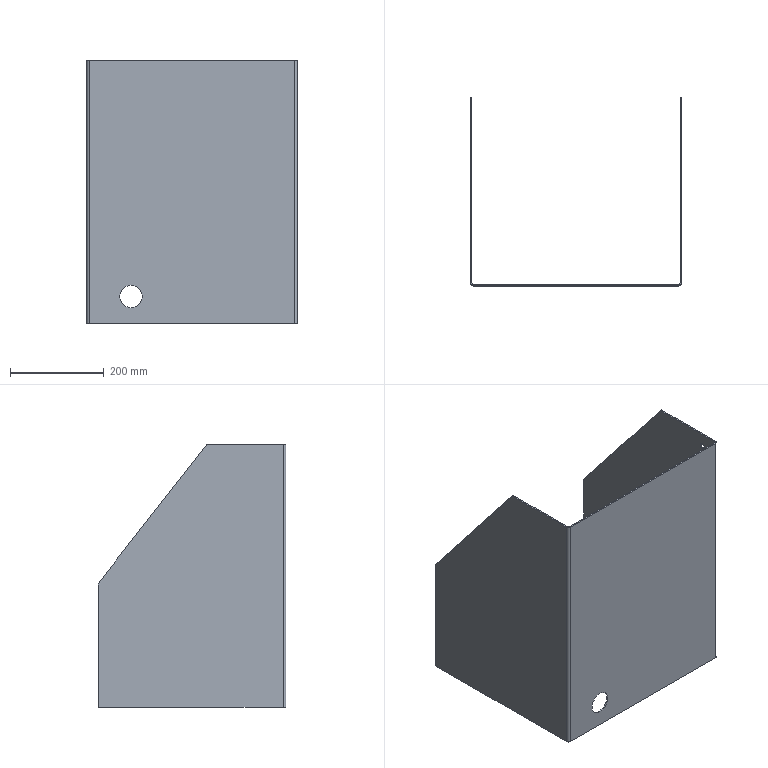Part | SolidWorks | features ICE 2, Cut 1, FlatPattern 1, SMBaseFlange 1, SheetMetal 1 | 1 solid | 36 faces | box 450 x 401 x 560 mm | volume 1875203 mm3 | plane 20 | cylinder 16 | commonest cylinder face diameters 6 x8 12.5 x4 12 x2 48 x2
STEP:
#1=CARTESIAN_POINT('',(95.,3.,33.));
#2=VERTEX_POINT('',#1);
#3=CARTESIAN_POINT('',(95.,3.,81.));
#4=VERTEX_POINT('',#3);
#5=CARTESIAN_POINT('',(95.,3.,57.));
#6=DIRECTION('',(0.,1.,0.));
#7=DIRECTION('',(0.,0.,1.));
#8=AXIS2_PLACEMENT_3D('',#5,#6,#7);
#9=CIRCLE('',#8,24.);
#10=EDGE_CURVE('',#2,#4,#9,.T.);
#11=ORIENTED_EDGE('',*,*,#10,.T.);
#12=CARTESIAN_POINT('',(95.,0.,81.));
#13=VERTEX_POINT('',#12);
#14=CARTESIAN_POINT('',(95.,10.,81.));
#15=DIRECTION('',(0.,-1.,0.));
#16=VECTOR('',#15,1000.);
#17=LINE('',#14,#16);
#18=EDGE_CURVE('',#4,#13,#17,.T.);
#19=ORIENTED_EDGE('',*,*,#18,.T.);
#20=CARTESIAN_POINT('',(95.,0.,33.));
#21=VERTEX_POINT('',#20);
#22=CARTESIAN_POINT('',(95.,0.,57.));
#23=DIRECTION('',(0.,-1.,0.));
#24=DIRECTION('',(0.,0.,-1.));
#25=AXIS2_PLACEMENT_3D('',#22,#23,#24);
#26=CIRCLE('',#25,24.);
#27=EDGE_CURVE('',#13,#21,#26,.T.);
#28=ORIENTED_EDGE('',*,*,#27,.T.);
#29=CARTESIAN_POINT('',(95.,10.,33.));
#30=DIRECTION('',(0.,-1.,0.));
#31=VECTOR('',#30,1000.);
#32=LINE('',#29,#31);
#33=EDGE_CURVE('',#2,#21,#32,.T.);
#34=ORIENTED_EDGE('',*,*,#33,.F.);
#35=EDGE_LOOP('',(#11,#19,#28,#34));
#36=FACE_OUTER_BOUND('',#35,.T.);
#37=CARTESIAN_POINT('',(95.,10.,57.));
#38=DIRECTION('',(0.,-1.,0.));
#39=DIRECTION('',(0.,0.,-1.));
#40=AXIS2_PLACEMENT_3D('',#37,#38,#39);
#41=CYLINDRICAL_SURFACE('',#40,24.);
#42=ADVANCED_FACE('',(#36),#41,.F.);
#43=CARTESIAN_POINT('',(447.,43.,373.75));
#44=VERTEX_POINT('',#43);
#45=CARTESIAN_POINT('',(447.,43.,386.25));
#46=VERTEX_POINT('',#45);
#47=CARTESIAN_POINT('',(447.,43.,380.));
#48=DIRECTION('',(-1.,0.,0.));
#49=DIRECTION('',(0.,0.,1.));
#50=AXIS2_PLACEMENT_3D('',#47,#48,#49);
#51=CIRCLE('',#50,6.25);
#52=EDGE_CURVE('',#44,#46,#51,.T.);
#53=ORIENTED_EDGE('',*,*,#52,.T.);
#54=CARTESIAN_POINT('',(450.,43.,386.25));
#55=VERTEX_POINT('',#54);
#56=CARTESIAN_POINT('',(440.,43.,386.25));
#57=DIRECTION('',(1.,0.,0.));
#58=VECTOR('',#57,1000.);
#59=LINE('',#56,#58);
#60=EDGE_CURVE('',#46,#55,#59,.T.);
#61=ORIENTED_EDGE('',*,*,#60,.T.);
#62=CARTESIAN_POINT('',(450.,43.,373.75));
#63=VERTEX_POINT('',#62);
#64=CARTESIAN_POINT('',(450.,43.,380.));
#65=DIRECTION('',(1.,0.,0.));
#66=DIRECTION('',(0.,0.,-1.));
#67=AXIS2_PLACEMENT_3D('',#64,#65,#66);
#68=CIRCLE('',#67,6.25);
#69=EDGE_CURVE('',#55,#63,#68,.T.);
#70=ORIENTED_EDGE('',*,*,#69,.T.);
#71=CARTESIAN_POINT('',(440.,43.,373.75));
#72=DIRECTION('',(1.,0.,0.));
#73=VECTOR('',#72,1000.);
#74=LINE('',#71,#73);
#75=EDGE_CURVE('',#44,#63,#74,.T.);
#76=ORIENTED_EDGE('',*,*,#75,.F.);
#77=EDGE_LOOP('',(#53,#61,#70,#76));
#78=FACE_OUTER_BOUND('',#77,.T.);
#79=CARTESIAN_POINT('',(440.,43.,380.));
#80=DIRECTION('',(1.,0.,0.));
#81=DIRECTION('',(0.,0.,-1.));
#82=AXIS2_PLACEMENT_3D('',#79,#80,#81);
#83=CYLINDRICAL_SURFACE('',#82,6.25);
#84=ADVANCED_FACE('',(#78),#83,.F.);
#85=CARTESIAN_POINT('',(447.,43.,523.75));
#86=VERTEX_POINT('',#85);
#87=CARTESIAN_POINT('',(447.,43.,536.25));
#88=VERTEX_POINT('',#87);
#89=CARTESIAN_POINT('',(447.,43.,530.));
#90=DIRECTION('',(-1.,0.,0.));
#91=DIRECTION('',(0.,0.,1.));
#92=AXIS2_PLACEMENT_3D('',#89,#90,#91);
#93=CIRCLE('',#92,6.25);
#94=EDGE_CURVE('',#86,#88,#93,.T.);
#95=ORIENTED_EDGE('',*,*,#94,.T.);
#96=CARTESIAN_POINT('',(450.,43.,536.25));
#97=VERTEX_POINT('',#96);
#98=CARTESIAN_POINT('',(440.,43.,536.25));
#99=DIRECTION('',(1.,0.,0.));
#100=VECTOR('',#99,1000.);
#101=LINE('',#98,#100);
#102=EDGE_CURVE('',#88,#97,#101,.T.);
#103=ORIENTED_EDGE('',*,*,#102,.T.);
#104=CARTESIAN_POINT('',(450.,43.,523.75));
#105=VERTEX_POINT('',#104);
#106=CARTESIAN_POINT('',(450.,43.,530.));
#107=DIRECTION('',(1.,0.,0.));
#108=DIRECTION('',(0.,0.,-1.));
#109=AXIS2_PLACEMENT_3D('',#106,#107,#108);
#110=CIRCLE('',#109,6.25);
#111=EDGE_CURVE('',#97,#105,#110,.T.);
#112=ORIENTED_EDGE('',*,*,#111,.T.);
#113=CARTESIAN_POINT('',(440.,43.,523.75));
#114=DIRECTION('',(1.,0.,0.));
#115=VECTOR('',#114,1000.);
#116=LINE('',#113,#115);
#117=EDGE_CURVE('',#86,#105,#116,.T.);
#118=ORIENTED_EDGE('',*,*,#117,.F.);
#119=EDGE_LOOP('',(#95,#103,#112,#118));
#120=FACE_OUTER_BOUND('',#119,.T.);
#121=CARTESIAN_POINT('',(440.,43.,530.));
#122=DIRECTION('',(1.,0.,0.));
#123=DIRECTION('',(0.,0.,-1.));
#124=AXIS2_PLACEMENT_3D('',#121,#122,#123);
#125=CYLINDRICAL_SURFACE('',#124,6.25);
#126=ADVANCED_FACE('',(#120),#125,.F.);
#127=CARTESIAN_POINT('',(450.,43.,380.));
#128=DIRECTION('',(1.,0.,0.));
#129=DIRECTION('',(0.,0.,-1.));
#130=AXIS2_PLACEMENT_3D('',#127,#128,#129);
#131=CIRCLE('',#130,6.25);
#132=EDGE_CURVE('',#63,#55,#131,.T.);
#133=ORIENTED_EDGE('',*,*,#132,.F.);
#134=ORIENTED_EDGE('',*,*,#69,.F.);
#135=EDGE_LOOP('',(#133,#134));
#136=FACE_BOUND('',#135,.T.);
#137=CARTESIAN_POINT('',(450.,43.,530.));
#138=DIRECTION('',(1.,0.,0.));
#139=DIRECTION('',(0.,0.,-1.));
#140=AXIS2_PLACEMENT_3D('',#137,#138,#139);
#141=CIRCLE('',#140,6.25);
#142=EDGE_CURVE('',#105,#97,#141,.T.);
#143=ORIENTED_EDGE('',*,*,#142,.F.);
#144=ORIENTED_EDGE('',*,*,#111,.F.);
#145=EDGE_LOOP('',(#143,#144));
#146=FACE_BOUND('',#145,.T.);
#147=CARTESIAN_POINT('',(450.,398.,0.));
#148=VERTEX_POINT('',#147);
#149=CARTESIAN_POINT('',(450.,401.,3.));
#150=VERTEX_POINT('',#149);
#151=CARTESIAN_POINT('',(450.,398.,3.));
#152=DIRECTION('',(1.,0.,0.));
#153=DIRECTION('',(0.,0.,1.));
#154=AXIS2_PLACEMENT_3D('',#151,#152,#153);
#155=CIRCLE('',#154,3.);
#156=EDGE_CURVE('',#148,#150,#155,.T.);
#157=ORIENTED_EDGE('',*,*,#156,.T.);
#158=CARTESIAN_POINT('',(450.,401.,262.934));
#159=VERTEX_POINT('',#158);
#160=CARTESIAN_POINT('',(450.,401.,560.));
#161=DIRECTION('',(0.,0.,-1.));
#162=VECTOR('',#161,1000.);
#163=LINE('',#160,#162);
#164=EDGE_CURVE('',#159,#150,#163,.T.);
#165=ORIENTED_EDGE('',*,*,#164,.F.);
#166=CARTESIAN_POINT('',(450.,400.364,264.781));
#167=VERTEX_POINT('',#166);
#168=CARTESIAN_POINT('',(450.,398.,262.934));
#169=DIRECTION('',(1.,0.,0.));
#170=DIRECTION('',(0.,0.,1.));
#171=AXIS2_PLACEMENT_3D('',#168,#169,#170);
#172=CIRCLE('',#171,3.);
#173=EDGE_CURVE('',#159,#167,#172,.T.);
#174=ORIENTED_EDGE('',*,*,#173,.T.);
#175=CARTESIAN_POINT('',(450.,170.611,558.847));
#176=VERTEX_POINT('',#175);
#177=CARTESIAN_POINT('',(450.,105.382,642.335));
#178=DIRECTION('',(0.,-0.6157,0.788));
#179=VECTOR('',#178,1000.);
#180=LINE('',#177,#179);
#181=EDGE_CURVE('',#167,#176,#180,.T.);
#182=ORIENTED_EDGE('',*,*,#181,.T.);
#183=CARTESIAN_POINT('',(450.,168.247,560.));
#184=VERTEX_POINT('',#183);
#185=CARTESIAN_POINT('',(450.,168.247,557.));
#186=DIRECTION('',(1.,0.,0.));
#187=DIRECTION('',(0.,0.,1.));
#188=AXIS2_PLACEMENT_3D('',#185,#186,#187);
#189=CIRCLE('',#188,3.);
#190=EDGE_CURVE('',#176,#184,#189,.T.);
#191=ORIENTED_EDGE('',*,*,#190,.T.);
#192=CARTESIAN_POINT('',(450.,6.,560.));
#193=VERTEX_POINT('',#192);
#194=CARTESIAN_POINT('',(450.,0.,560.));
#195=DIRECTION('',(0.,1.,0.));
#196=VECTOR('',#195,1000.);
#197=LINE('',#194,#196);
#198=EDGE_CURVE('',#193,#184,#197,.T.);
#199=ORIENTED_EDGE('',*,*,#198,.F.);
#200=CARTESIAN_POINT('',(450.,6.,0.));
#201=VERTEX_POINT('',#200);
#202=CARTESIAN_POINT('',(450.,6.,560.));
#203=DIRECTION('',(0.,0.,-1.));
#204=VECTOR('',#203,1000.);
#205=LINE('',#202,#204);
#206=EDGE_CURVE('',#193,#201,#205,.T.);
#207=ORIENTED_EDGE('',*,*,#206,.T.);
#208=CARTESIAN_POINT('',(450.,0.,0.));
#209=DIRECTION('',(0.,1.,0.));
#210=VECTOR('',#209,1000.);
#211=LINE('',#208,#210);
#212=EDGE_CURVE('',#201,#148,#211,.T.);
#213=ORIENTED_EDGE('',*,*,#212,.T.);
#214=EDGE_LOOP('',(#157,#165,#174,#182,#191,#199,#207,#213));
#215=FACE_OUTER_BOUND('',#214,.T.);
#216=CARTESIAN_POINT('',(450.,0.,560.));
#217=DIRECTION('',(-1.,0.,0.));
#218=DIRECTION('',(0.,0.,1.));
#219=AXIS2_PLACEMENT_3D('',#216,#217,#218);
#220=PLANE('',#219);
#221=ADVANCED_FACE('',(#136,#146,#215),#220,.F.);
#222=ORIENTED_EDGE('',*,*,#52,.F.);
#223=CARTESIAN_POINT('',(447.,43.,380.));
#224=DIRECTION('',(-1.,0.,0.));
#225=DIRECTION('',(0.,0.,1.));
#226=AXIS2_PLACEMENT_3D('',#223,#224,#225);
#227=CIRCLE('',#226,6.25);
#228=EDGE_CURVE('',#46,#44,#227,.T.);
#229=ORIENTED_EDGE('',*,*,#228,.F.);
#230=EDGE_LOOP('',(#222,#229));
#231=FACE_BOUND('',#230,.T.);
#232=ORIENTED_EDGE('',*,*,#94,.F.);
#233=CARTESIAN_POINT('',(447.,43.,530.));
#234=DIRECTION('',(-1.,0.,0.));
#235=DIRECTION('',(0.,0.,1.));
#236=AXIS2_PLACEMENT_3D('',#233,#234,#235);
#237=CIRCLE('',#236,6.25);
#238=EDGE_CURVE('',#88,#86,#237,.T.);
#239=ORIENTED_EDGE('',*,*,#238,.F.);
#240=EDGE_LOOP('',(#232,#239));
#241=FACE_BOUND('',#240,.T.);
#242=CARTESIAN_POINT('',(447.,401.,262.934));
#243=VERTEX_POINT('',#242);
#244=CARTESIAN_POINT('',(447.,401.,3.));
#245=VERTEX_POINT('',#244);
#246=CARTESIAN_POINT('',(447.,401.,560.));
#247=DIRECTION('',(0.,0.,-1.));
#248=VECTOR('',#247,1000.);
#249=LINE('',#246,#248);
#250=EDGE_CURVE('',#243,#245,#249,.T.);
#251=ORIENTED_EDGE('',*,*,#250,.T.);
#252=CARTESIAN_POINT('',(447.,398.,0.));
#253=VERTEX_POINT('',#252);
#254=CARTESIAN_POINT('',(447.,398.,3.));
#255=DIRECTION('',(1.,0.,0.));
#256=DIRECTION('',(0.,0.,1.));
#257=AXIS2_PLACEMENT_3D('',#254,#255,#256);
#258=CIRCLE('',#257,3.);
#259=EDGE_CURVE('',#253,#245,#258,.T.);
#260=ORIENTED_EDGE('',*,*,#259,.F.);
#261=CARTESIAN_POINT('',(447.,6.,0.));
#262=VERTEX_POINT('',#261);
#263=CARTESIAN_POINT('',(447.,0.,0.));
#264=DIRECTION('',(0.,1.,0.));
#265=VECTOR('',#264,1000.);
#266=LINE('',#263,#265);
#267=EDGE_CURVE('',#262,#253,#266,.T.);
#268=ORIENTED_EDGE('',*,*,#267,.F.);
#269=CARTESIAN_POINT('',(447.,6.,560.));
#270=VERTEX_POINT('',#269);
#271=CARTESIAN_POINT('',(447.,6.,560.));
#272=DIRECTION('',(0.,0.,-1.));
#273=VECTOR('',#272,1000.);
#274=LINE('',#271,#273);
#275=EDGE_CURVE('',#270,#262,#274,.T.);
#276=ORIENTED_EDGE('',*,*,#275,.F.);
#277=CARTESIAN_POINT('',(447.,168.247,560.));
#278=VERTEX_POINT('',#277);
#279=CARTESIAN_POINT('',(447.,0.,560.));
#280=DIRECTION('',(0.,1.,0.));
#281=VECTOR('',#280,1000.);
#282=LINE('',#279,#281);
#283=EDGE_CURVE('',#270,#278,#282,.T.);
#284=ORIENTED_EDGE('',*,*,#283,.T.);
#285=CARTESIAN_POINT('',(447.,170.611,558.847));
#286=VERTEX_POINT('',#285);
#287=CARTESIAN_POINT('',(447.,168.247,557.));
#288=DIRECTION('',(1.,0.,0.));
#289=DIRECTION('',(0.,0.,1.));
#290=AXIS2_PLACEMENT_3D('',#287,#288,#289);
#291=CIRCLE('',#290,3.);
#292=EDGE_CURVE('',#286,#278,#291,.T.);
#293=ORIENTED_EDGE('',*,*,#292,.F.);
#294=CARTESIAN_POINT('',(447.,400.364,264.781));
#295=VERTEX_POINT('',#294);
#296=CARTESIAN_POINT('',(447.,105.382,642.335));
#297=DIRECTION('',(0.,-0.6157,0.788));
#298=VECTOR('',#297,1000.);
#299=LINE('',#296,#298);
#300=EDGE_CURVE('',#295,#286,#299,.T.);
#301=ORIENTED_EDGE('',*,*,#300,.F.);
#302=CARTESIAN_POINT('',(447.,398.,262.934));
#303=DIRECTION('',(1.,0.,0.));
#304=DIRECTION('',(0.,0.,1.));
#305=AXIS2_PLACEMENT_3D('',#302,#303,#304);
#306=CIRCLE('',#305,3.);
#307=EDGE_CURVE('',#243,#295,#306,.T.);
#308=ORIENTED_EDGE('',*,*,#307,.F.);
#309=EDGE_LOOP('',(#251,#260,#268,#276,#284,#293,#301,#308));
#310=FACE_OUTER_BOUND('',#309,.T.);
#311=CARTESIAN_POINT('',(447.,0.,560.));
#312=DIRECTION('',(-1.,0.,0.));
#313=DIRECTION('',(0.,0.,1.));
#314=AXIS2_PLACEMENT_3D('',#311,#312,#313);
#315=PLANE('',#314);
#316=ADVANCED_FACE('',(#231,#241,#310),#315,.T.);
#317=ORIENTED_EDGE('',*,*,#164,.T.);
#318=CARTESIAN_POINT('',(447.,401.,3.));
#319=DIRECTION('',(1.,0.,0.));
#320=VECTOR('',#319,1000.);
#321=LINE('',#318,#320);
#322=EDGE_CURVE('',#245,#150,#321,.T.);
#323=ORIENTED_EDGE('',*,*,#322,.F.);
#324=ORIENTED_EDGE('',*,*,#250,.F.);
#325=CARTESIAN_POINT('',(447.,401.,262.934));
#326=DIRECTION('',(1.,0.,0.));
#327=VECTOR('',#326,1000.);
#328=LINE('',#325,#327);
#329=EDGE_CURVE('',#243,#159,#328,.T.);
#330=ORIENTED_EDGE('',*,*,#329,.T.);
#331=EDGE_LOOP('',(#317,#323,#324,#330));
#332=FACE_OUTER_BOUND('',#331,.T.);
#333=CARTESIAN_POINT('',(447.,401.,560.));
#334=DIRECTION('',(0.,1.,0.));
#335=DIRECTION('',(0.,0.,1.));
#336=AXIS2_PLACEMENT_3D('',#333,#334,#335);
#337=PLANE('',#336);
#338=ADVANCED_FACE('',(#332),#337,.T.);
#339=CARTESIAN_POINT('',(3.,398.,0.));
#340=VERTEX_POINT('',#339);
#341=CARTESIAN_POINT('',(3.,6.,0.));
#342=VERTEX_POINT('',#341);
#343=CARTESIAN_POINT('',(3.,0.,0.));
#344=DIRECTION('',(0.,-1.,0.));
#345=VECTOR('',#344,1000.);
#346=LINE('',#343,#345);
#347=EDGE_CURVE('',#340,#342,#346,.T.);
#348=ORIENTED_EDGE('',*,*,#347,.F.);
#349=CARTESIAN_POINT('',(3.,401.,3.));
#350=VERTEX_POINT('',#349);
#351=CARTESIAN_POINT('',(3.,398.,3.));
#352=DIRECTION('',(-1.,0.,0.));
#353=DIRECTION('',(0.,0.,-1.));
#354=AXIS2_PLACEMENT_3D('',#351,#352,#353);
#355=CIRCLE('',#354,3.);
#356=EDGE_CURVE('',#350,#340,#355,.T.);
#357=ORIENTED_EDGE('',*,*,#356,.F.);
#358=CARTESIAN_POINT('',(3.,401.,262.934));
#359=VERTEX_POINT('',#358);
#360=CARTESIAN_POINT('',(3.,401.,560.));
#361=DIRECTION('',(0.,0.,-1.));
#362=VECTOR('',#361,1000.);
#363=LINE('',#360,#362);
#364=EDGE_CURVE('',#359,#350,#363,.T.);
#365=ORIENTED_EDGE('',*,*,#364,.F.);
#366=CARTESIAN_POINT('',(3.,400.364,264.781));
#367=VERTEX_POINT('',#366);
#368=CARTESIAN_POINT('',(3.,398.,262.934));
#369=DIRECTION('',(-1.,0.,0.));
#370=DIRECTION('',(0.,0.,-1.));
#371=AXIS2_PLACEMENT_3D('',#368,#369,#370);
#372=CIRCLE('',#371,3.);
#373=EDGE_CURVE('',#367,#359,#372,.T.);
#374=ORIENTED_EDGE('',*,*,#373,.F.);
#375=CARTESIAN_POINT('',(3.,170.611,558.847));
#376=VERTEX_POINT('',#375);
#377=CARTESIAN_POINT('',(3.,105.382,642.335));
#378=DIRECTION('',(0.,0.6157,-0.788));
#379=VECTOR('',#378,1000.);
#380=LINE('',#377,#379);
#381=EDGE_CURVE('',#376,#367,#380,.T.);
#382=ORIENTED_EDGE('',*,*,#381,.F.);
#383=CARTESIAN_POINT('',(3.,168.247,560.));
#384=VERTEX_POINT('',#383);
#385=CARTESIAN_POINT('',(3.,168.247,557.));
#386=DIRECTION('',(-1.,0.,0.));
#387=DIRECTION('',(0.,0.,-1.));
#388=AXIS2_PLACEMENT_3D('',#385,#386,#387);
#389=CIRCLE('',#388,3.);
#390=EDGE_CURVE('',#384,#376,#389,.T.);
#391=ORIENTED_EDGE('',*,*,#390,.F.);
#392=CARTESIAN_POINT('',(3.,6.,560.));
#393=VERTEX_POINT('',#392);
#394=CARTESIAN_POINT('',(3.,0.,560.));
#395=DIRECTION('',(0.,-1.,0.));
#396=VECTOR('',#395,1000.);
#397=LINE('',#394,#396);
#398=EDGE_CURVE('',#384,#393,#397,.T.);
#399=ORIENTED_EDGE('',*,*,#398,.T.);
#400=CARTESIAN_POINT('',(3.,6.,560.));
#401=DIRECTION('',(0.,0.,-1.));
#402=VECTOR('',#401,1000.);
#403=LINE('',#400,#402);
#404=EDGE_CURVE('',#393,#342,#403,.T.);
#405=ORIENTED_EDGE('',*,*,#404,.T.);
#406=EDGE_LOOP('',(#348,#357,#365,#374,#382,#391,#399,#405));
#407=FACE_OUTER_BOUND('',#406,.T.);
#408=CARTESIAN_POINT('',(3.,0.,560.));
#409=DIRECTION('',(1.,0.,0.));
#410=DIRECTION('',(0.,0.,-1.));
#411=AXIS2_PLACEMENT_3D('',#408,#409,#410);
#412=PLANE('',#411);
#413=ADVANCED_FACE('',(#407),#412,.T.);
#414=CARTESIAN_POINT('',(0.,401.,3.));
#415=VERTEX_POINT('',#414);
#416=CARTESIAN_POINT('',(0.,398.,0.));
#417=VERTEX_POINT('',#416);
#418=CARTESIAN_POINT('',(0.,398.,3.));
#419=DIRECTION('',(-1.,0.,0.));
#420=DIRECTION('',(0.,0.,-1.));
#421=AXIS2_PLACEMENT_3D('',#418,#419,#420);
#422=CIRCLE('',#421,3.);
#423=EDGE_CURVE('',#415,#417,#422,.T.);
#424=ORIENTED_EDGE('',*,*,#423,.T.);
#425=CARTESIAN_POINT('',(0.,6.,0.));
#426=VERTEX_POINT('',#425);
#427=CARTESIAN_POINT('',(0.,0.,0.));
#428=DIRECTION('',(0.,-1.,0.));
#429=VECTOR('',#428,1000.);
#430=LINE('',#427,#429);
#431=EDGE_CURVE('',#417,#426,#430,.T.);
#432=ORIENTED_EDGE('',*,*,#431,.T.);
#433=CARTESIAN_POINT('',(0.,6.,560.));
#434=VERTEX_POINT('',#433);
#435=CARTESIAN_POINT('',(0.,6.,560.));
#436=DIRECTION('',(0.,0.,-1.));
#437=VECTOR('',#436,1000.);
#438=LINE('',#435,#437);
#439=EDGE_CURVE('',#434,#426,#438,.T.);
#440=ORIENTED_EDGE('',*,*,#439,.F.);
#441=CARTESIAN_POINT('',(0.,168.247,560.));
#442=VERTEX_POINT('',#441);
#443=CARTESIAN_POINT('',(0.,0.,560.));
#444=DIRECTION('',(0.,-1.,0.));
#445=VECTOR('',#444,1000.);
#446=LINE('',#443,#445);
#447=EDGE_CURVE('',#442,#434,#446,.T.);
#448=ORIENTED_EDGE('',*,*,#447,.F.);
#449=CARTESIAN_POINT('',(0.,170.611,558.847));
#450=VERTEX_POINT('',#449);
#451=CARTESIAN_POINT('',(0.,168.247,557.));
#452=DIRECTION('',(-1.,0.,0.));
#453=DIRECTION('',(0.,0.,-1.));
#454=AXIS2_PLACEMENT_3D('',#451,#452,#453);
#455=CIRCLE('',#454,3.);
#456=EDGE_CURVE('',#442,#450,#455,.T.);
#457=ORIENTED_EDGE('',*,*,#456,.T.);
#458=CARTESIAN_POINT('',(0.,400.364,264.781));
#459=VERTEX_POINT('',#458);
#460=CARTESIAN_POINT('',(0.,105.382,642.335));
#461=DIRECTION('',(0.,0.6157,-0.788));
#462=VECTOR('',#461,1000.);
#463=LINE('',#460,#462);
#464=EDGE_CURVE('',#450,#459,#463,.T.);
#465=ORIENTED_EDGE('',*,*,#464,.T.);
#466=CARTESIAN_POINT('',(0.,401.,262.934));
#467=VERTEX_POINT('',#466);
#468=CARTESIAN_POINT('',(0.,398.,262.934));
#469=DIRECTION('',(-1.,0.,0.));
#470=DIRECTION('',(0.,0.,-1.));
#471=AXIS2_PLACEMENT_3D('',#468,#469,#470);
#472=CIRCLE('',#471,3.);
#473=EDGE_CURVE('',#459,#467,#472,.T.);
#474=ORIENTED_EDGE('',*,*,#473,.T.);
#475=CARTESIAN_POINT('',(0.,401.,560.));
#476=DIRECTION('',(0.,0.,-1.));
#477=VECTOR('',#476,1000.);
#478=LINE('',#475,#477);
#479=EDGE_CURVE('',#467,#415,#478,.T.);
#480=ORIENTED_EDGE('',*,*,#479,.T.);
#481=EDGE_LOOP('',(#424,#432,#440,#448,#457,#465,#474,#480));
#482=FACE_OUTER_BOUND('',#481,.T.);
#483=CARTESIAN_POINT('',(0.,0.,560.));
#484=DIRECTION('',(1.,0.,0.));
#485=DIRECTION('',(0.,0.,-1.));
#486=AXIS2_PLACEMENT_3D('',#483,#484,#485);
#487=PLANE('',#486);
#488=ADVANCED_FACE('',(#482),#487,.F.);
#489=ORIENTED_EDGE('',*,*,#198,.T.);
#490=CARTESIAN_POINT('',(447.,168.247,560.));
#491=DIRECTION('',(1.,0.,0.));
#492=VECTOR('',#491,1000.);
#493=LINE('',#490,#492);
#494=EDGE_CURVE('',#278,#184,#493,.T.);
#495=ORIENTED_EDGE('',*,*,#494,.F.);
#496=ORIENTED_EDGE('',*,*,#283,.F.);
#497=CARTESIAN_POINT('',(447.,6.,560.));
#498=DIRECTION('',(1.,0.,0.));
#499=VECTOR('',#498,1000.);
#500=LINE('',#497,#499);
#501=EDGE_CURVE('',#270,#193,#500,.T.);
#502=ORIENTED_EDGE('',*,*,#501,.T.);
#503=EDGE_LOOP('',(#489,#495,#496,#502));
#504=FACE_OUTER_BOUND('',#503,.T.);
#505=CARTESIAN_POINT('',(444.,6.,560.));
#506=DIRECTION('',(0.,0.,1.));
#507=DIRECTION('',(1.,0.,0.));
#508=AXIS2_PLACEMENT_3D('',#505,#506,#507);
#509=PLANE('',#508);
#510=ADVANCED_FACE('',(#504),#509,.T.);
#511=CARTESIAN_POINT('',(3.,401.,3.));
#512=DIRECTION('',(-1.,0.,0.));
#513=VECTOR('',#512,1000.);
#514=LINE('',#511,#513);
#515=EDGE_CURVE('',#350,#415,#514,.T.);
#516=ORIENTED_EDGE('',*,*,#515,.T.);
#517=ORIENTED_EDGE('',*,*,#479,.F.);
#518=CARTESIAN_POINT('',(3.,401.,262.934));
#519=DIRECTION('',(-1.,0.,0.));
#520=VECTOR('',#519,1000.);
#521=LINE('',#518,#520);
#522=EDGE_CURVE('',#359,#467,#521,.T.);
#523=ORIENTED_EDGE('',*,*,#522,.F.);
#524=ORIENTED_EDGE('',*,*,#364,.T.);
#525=EDGE_LOOP('',(#516,#517,#523,#524));
#526=FACE_OUTER_BOUND('',#525,.T.);
#527=CARTESIAN_POINT('',(0.,401.,560.));
#528=DIRECTION('',(0.,1.,0.));
#529=DIRECTION('',(0.,0.,1.));
#530=AXIS2_PLACEMENT_3D('',#527,#528,#529);
#531=PLANE('',#530);
#532=ADVANCED_FACE('',(#526),#531,.T.);
#533=CARTESIAN_POINT('',(0.,6.,560.));
#534=DIRECTION('',(1.,0.,0.));
#535=VECTOR('',#534,1000.);
#536=LINE('',#533,#535);
#537=EDGE_CURVE('',#434,#393,#536,.T.);
#538=ORIENTED_EDGE('',*,*,#537,.F.);
#539=CARTESIAN_POINT('',(6.,0.,560.));
#540=VERTEX_POINT('',#539);
#541=CARTESIAN_POINT('',(6.,6.,560.));
#542=DIRECTION('',(0.,0.,1.));
#543=DIRECTION('',(-1.,0.,0.));
#544=AXIS2_PLACEMENT_3D('',#541,#542,#543);
#545=CIRCLE('',#544,6.);
#546=EDGE_CURVE('',#434,#540,#545,.T.);
#547=ORIENTED_EDGE('',*,*,#546,.T.);
#548=CARTESIAN_POINT('',(6.,3.,560.));
#549=VERTEX_POINT('',#548);
#550=CARTESIAN_POINT('',(6.,3.,560.));
#551=DIRECTION('',(0.,-1.,0.));
#552=VECTOR('',#551,1000.);
#553=LINE('',#550,#552);
#554=EDGE_CURVE('',#549,#540,#553,.T.);
#555=ORIENTED_EDGE('',*,*,#554,.F.);
#556=CARTESIAN_POINT('',(6.,6.,560.));
#557=DIRECTION('',(0.,0.,1.));
#558=DIRECTION('',(1.,0.,0.));
#559=AXIS2_PLACEMENT_3D('',#556,#557,#558);
#560=CIRCLE('',#559,3.);
#561=EDGE_CURVE('',#393,#549,#560,.T.);
#562=ORIENTED_EDGE('',*,*,#561,.F.);
#563=EDGE_LOOP('',(#538,#547,#555,#562));
#564=FACE_OUTER_BOUND('',#563,.T.);
#565=CARTESIAN_POINT('',(0.,6.,560.));
#566=DIRECTION('',(0.,0.,1.));
#567=DIRECTION('',(1.,0.,0.));
#568=AXIS2_PLACEMENT_3D('',#565,#566,#567);
#569=PLANE('',#568);
#570=ADVANCED_FACE('',(#564),#569,.T.);
#571=CARTESIAN_POINT('',(3.,168.247,560.));
#572=DIRECTION('',(-1.,0.,0.));
#573=VECTOR('',#572,1000.);
#574=LINE('',#571,#573);
#575=EDGE_CURVE('',#384,#442,#574,.T.);
#576=ORIENTED_EDGE('',*,*,#575,.T.);
#577=ORIENTED_EDGE('',*,*,#447,.T.);
#578=ORIENTED_EDGE('',*,*,#537,.T.);
#579=ORIENTED_EDGE('',*,*,#398,.F.);
#580=EDGE_LOOP('',(#576,#577,#578,#579));
#581=FACE_OUTER_BOUND('',#580,.T.);
#582=CARTESIAN_POINT('',(6.,3.,560.));
#583=DIRECTION('',(0.,0.,1.));
#584=DIRECTION('',(1.,0.,0.));
#585=AXIS2_PLACEMENT_3D('',#582,#583,#584);
#586=PLANE('',#585);
#587=ADVANCED_FACE('',(#581),#586,.T.);
#588=CARTESIAN_POINT('',(6.,0.,0.));
#589=VERTEX_POINT('',#588);
#590=CARTESIAN_POINT('',(6.,3.,0.));
#591=VERTEX_POINT('',#590);
#592=CARTESIAN_POINT('',(6.,0.,0.));
#593=DIRECTION('',(0.,1.,0.));
#594=VECTOR('',#593,1000.);
#595=LINE('',#592,#594);
#596=EDGE_CURVE('',#589,#591,#595,.T.);
#597=ORIENTED_EDGE('',*,*,#596,.F.);
#598=CARTESIAN_POINT('',(6.,6.,0.));
#599=DIRECTION('',(0.,0.,1.));
#600=DIRECTION('',(-1.,0.,0.));
#601=AXIS2_PLACEMENT_3D('',#598,#599,#600);
#602=CIRCLE('',#601,6.);
#603=EDGE_CURVE('',#426,#589,#602,.T.);
#604=ORIENTED_EDGE('',*,*,#603,.F.);
#605=CARTESIAN_POINT('',(3.,6.,0.));
#606=DIRECTION('',(-1.,0.,0.));
#607=VECTOR('',#606,1000.);
#608=LINE('',#605,#607);
#609=EDGE_CURVE('',#342,#426,#608,.T.);
#610=ORIENTED_EDGE('',*,*,#609,.F.);
#611=CARTESIAN_POINT('',(6.,6.,0.));
#612=DIRECTION('',(0.,0.,1.));
#613=DIRECTION('',(1.,0.,0.));
#614=AXIS2_PLACEMENT_3D('',#611,#612,#613);
#615=CIRCLE('',#614,3.);
#616=EDGE_CURVE('',#342,#591,#615,.T.);
#617=ORIENTED_EDGE('',*,*,#616,.T.);
#618=EDGE_LOOP('',(#597,#604,#610,#617));
#619=FACE_OUTER_BOUND('',#618,.T.);
#620=CARTESIAN_POINT('',(6.,0.,0.));
#621=DIRECTION('',(0.,0.,-1.));
#622=DIRECTION('',(-1.,0.,0.));
#623=AXIS2_PLACEMENT_3D('',#620,#621,#622);
#624=PLANE('',#623);
#625=ADVANCED_FACE('',(#619),#624,.T.);
#626=CARTESIAN_POINT('',(444.,0.,0.));
#627=VERTEX_POINT('',#626);
#628=CARTESIAN_POINT('',(0.,0.,0.));
#629=DIRECTION('',(1.,0.,0.));
#630=VECTOR('',#629,1000.);
#631=LINE('',#628,#630);
#632=EDGE_CURVE('',#589,#627,#631,.T.);
#633=ORIENTED_EDGE('',*,*,#632,.F.);
#634=ORIENTED_EDGE('',*,*,#596,.T.);
#635=CARTESIAN_POINT('',(444.,3.,0.));
#636=VERTEX_POINT('',#635);
#637=CARTESIAN_POINT('',(0.,3.,0.));
#638=DIRECTION('',(1.,0.,0.));
#639=VECTOR('',#638,1000.);
#640=LINE('',#637,#639);
#641=EDGE_CURVE('',#591,#636,#640,.T.);
#642=ORIENTED_EDGE('',*,*,#641,.T.);
#643=CARTESIAN_POINT('',(444.,3.,0.));
#644=DIRECTION('',(0.,-1.,0.));
#645=VECTOR('',#644,1000.);
#646=LINE('',#643,#645);
#647=EDGE_CURVE('',#636,#627,#646,.T.);
#648=ORIENTED_EDGE('',*,*,#647,.T.);
#649=EDGE_LOOP('',(#633,#634,#642,#648));
#650=FACE_OUTER_BOUND('',#649,.T.);
#651=CARTESIAN_POINT('',(3.,6.,0.));
#652=DIRECTION('',(0.,0.,-1.));
#653=DIRECTION('',(-1.,0.,0.));
#654=AXIS2_PLACEMENT_3D('',#651,#652,#653);
#655=PLANE('',#654);
#656=ADVANCED_FACE('',(#650),#655,.T.);
#657=CARTESIAN_POINT('',(444.,0.,560.));
#658=VERTEX_POINT('',#657);
#659=CARTESIAN_POINT('',(444.,3.,560.));
#660=VERTEX_POINT('',#659);
#661=CARTESIAN_POINT('',(444.,0.,560.));
#662=DIRECTION('',(0.,1.,0.));
#663=VECTOR('',#662,1000.);
#664=LINE('',#661,#663);
#665=EDGE_CURVE('',#658,#660,#664,.T.);
#666=ORIENTED_EDGE('',*,*,#665,.F.);
#667=CARTESIAN_POINT('',(444.,6.,560.));
#668=DIRECTION('',(0.,0.,1.));
#669=DIRECTION('',(-1.,0.,0.));
#670=AXIS2_PLACEMENT_3D('',#667,#668,#669);
#671=CIRCLE('',#670,6.);
#672=EDGE_CURVE('',#658,#193,#671,.T.);
#673=ORIENTED_EDGE('',*,*,#672,.T.);
#674=ORIENTED_EDGE('',*,*,#501,.F.);
#675=CARTESIAN_POINT('',(444.,6.,560.));
#676=DIRECTION('',(0.,0.,1.));
#677=DIRECTION('',(1.,0.,0.));
#678=AXIS2_PLACEMENT_3D('',#675,#676,#677);
#679=CIRCLE('',#678,3.);
#680=EDGE_CURVE('',#660,#270,#679,.T.);
#681=ORIENTED_EDGE('',*,*,#680,.F.);
#682=EDGE_LOOP('',(#666,#673,#674,#681));
#683=FACE_OUTER_BOUND('',#682,.T.);
#684=CARTESIAN_POINT('',(444.,0.,560.));
#685=DIRECTION('',(0.,0.,1.));
#686=DIRECTION('',(1.,0.,0.));
#687=AXIS2_PLACEMENT_3D('',#684,#685,#686);
#688=PLANE('',#687);
#689=ADVANCED_FACE('',(#683),#688,.T.);
#690=CARTESIAN_POINT('',(0.,0.,560.));
#691=DIRECTION('',(1.,0.,0.));
#692=VECTOR('',#691,1000.);
#693=LINE('',#690,#692);
#694=EDGE_CURVE('',#540,#658,#693,.T.);
#695=ORIENTED_EDGE('',*,*,#694,.T.);
#696=ORIENTED_EDGE('',*,*,#665,.T.);
#697=CARTESIAN_POINT('',(0.,3.,560.));
#698=DIRECTION('',(1.,0.,0.));
#699=VECTOR('',#698,1000.);
#700=LINE('',#697,#699);
#701=EDGE_CURVE('',#549,#660,#700,.T.);
#702=ORIENTED_EDGE('',*,*,#701,.F.);
#703=ORIENTED_EDGE('',*,*,#554,.T.);
#704=EDGE_LOOP('',(#695,#696,#702,#703));
#705=FACE_OUTER_BOUND('',#704,.T.);
#706=CARTESIAN_POINT('',(447.,6.,560.));
#707=DIRECTION('',(0.,0.,1.));
#708=DIRECTION('',(1.,0.,0.));
#709=AXIS2_PLACEMENT_3D('',#706,#707,#708);
#710=PLANE('',#709);
#711=ADVANCED_FACE('',(#705),#710,.T.);
#712=CARTESIAN_POINT('',(450.,6.,0.));
#713=DIRECTION('',(-1.,0.,0.));
#714=VECTOR('',#713,1000.);
#715=LINE('',#712,#714);
#716=EDGE_CURVE('',#201,#262,#715,.T.);
#717=ORIENTED_EDGE('',*,*,#716,.F.);
#718=CARTESIAN_POINT('',(444.,6.,0.));
#719=DIRECTION('',(0.,0.,1.));
#720=DIRECTION('',(-1.,0.,0.));
#721=AXIS2_PLACEMENT_3D('',#718,#719,#720);
#722=CIRCLE('',#721,6.);
#723=EDGE_CURVE('',#627,#201,#722,.T.);
#724=ORIENTED_EDGE('',*,*,#723,.F.);
#725=ORIENTED_EDGE('',*,*,#647,.F.);
#726=CARTESIAN_POINT('',(444.,6.,0.));
#727=DIRECTION('',(0.,0.,1.));
#728=DIRECTION('',(1.,0.,0.));
#729=AXIS2_PLACEMENT_3D('',#726,#727,#728);
#730=CIRCLE('',#729,3.);
#731=EDGE_CURVE('',#636,#262,#730,.T.);
#732=ORIENTED_EDGE('',*,*,#731,.T.);
#733=EDGE_LOOP('',(#717,#724,#725,#732));
#734=FACE_OUTER_BOUND('',#733,.T.);
#735=CARTESIAN_POINT('',(450.,6.,0.));
#736=DIRECTION('',(0.,0.,-1.));
#737=DIRECTION('',(-1.,0.,0.));
#738=AXIS2_PLACEMENT_3D('',#735,#736,#737);
#739=PLANE('',#738);
#740=ADVANCED_FACE('',(#734),#739,.T.);
#741=CARTESIAN_POINT('',(447.,398.,0.));
#742=DIRECTION('',(1.,0.,0.));
#743=VECTOR('',#742,1000.);
#744=LINE('',#741,#743);
#745=EDGE_CURVE('',#253,#148,#744,.T.);
#746=ORIENTED_EDGE('',*,*,#745,.T.);
#747=ORIENTED_EDGE('',*,*,#212,.F.);
#748=ORIENTED_EDGE('',*,*,#716,.T.);
#749=ORIENTED_EDGE('',*,*,#267,.T.);
#750=EDGE_LOOP('',(#746,#747,#748,#749));
#751=FACE_OUTER_BOUND('',#750,.T.);
#752=CARTESIAN_POINT('',(444.,3.,0.));
#753=DIRECTION('',(0.,0.,-1.));
#754=DIRECTION('',(-1.,0.,0.));
#755=AXIS2_PLACEMENT_3D('',#752,#753,#754);
#756=PLANE('',#755);
#757=ADVANCED_FACE('',(#751),#756,.T.);
#758=ORIENTED_EDGE('',*,*,#731,.F.);
#759=CARTESIAN_POINT('',(444.,3.,560.));
#760=DIRECTION('',(0.,0.,-1.));
#761=VECTOR('',#760,1000.);
#762=LINE('',#759,#761);
#763=EDGE_CURVE('',#660,#636,#762,.T.);
#764=ORIENTED_EDGE('',*,*,#763,.F.);
#765=ORIENTED_EDGE('',*,*,#680,.T.);
#766=ORIENTED_EDGE('',*,*,#275,.T.);
#767=EDGE_LOOP('',(#758,#764,#765,#766));
#768=FACE_OUTER_BOUND('',#767,.T.);
#769=CARTESIAN_POINT('',(444.,6.,560.));
#770=DIRECTION('',(0.,0.,-1.));
#771=DIRECTION('',(-1.,0.,0.));
#772=AXIS2_PLACEMENT_3D('',#769,#770,#771);
#773=CYLINDRICAL_SURFACE('',#772,3.);
#774=ADVANCED_FACE('',(#768),#773,.F.);
#775=ORIENTED_EDGE('',*,*,#10,.F.);
#776=CARTESIAN_POINT('',(95.,3.,57.));
#777=DIRECTION('',(0.,1.,0.));
#778=DIRECTION('',(0.,0.,1.));
#779=AXIS2_PLACEMENT_3D('',#776,#777,#778);
#780=CIRCLE('',#779,24.);
#781=EDGE_CURVE('',#4,#2,#780,.T.);
#782=ORIENTED_EDGE('',*,*,#781,.F.);
#783=EDGE_LOOP('',(#775,#782));
#784=FACE_BOUND('',#783,.T.);
#785=ORIENTED_EDGE('',*,*,#641,.F.);
#786=CARTESIAN_POINT('',(6.,3.,560.));
#787=DIRECTION('',(0.,0.,-1.));
#788=VECTOR('',#787,1000.);
#789=LINE('',#786,#788);
#790=EDGE_CURVE('',#549,#591,#789,.T.);
#791=ORIENTED_EDGE('',*,*,#790,.F.);
#792=ORIENTED_EDGE('',*,*,#701,.T.);
#793=ORIENTED_EDGE('',*,*,#763,.T.);
#794=EDGE_LOOP('',(#785,#791,#792,#793));
#795=FACE_OUTER_BOUND('',#794,.T.);
#796=CARTESIAN_POINT('',(0.,3.,560.));
#797=DIRECTION('',(0.,1.,0.));
#798=DIRECTION('',(0.,0.,1.));
#799=AXIS2_PLACEMENT_3D('',#796,#797,#798);
#800=PLANE('',#799);
#801=ADVANCED_FACE('',(#784,#795),#800,.T.);
#802=ORIENTED_EDGE('',*,*,#616,.F.);
#803=ORIENTED_EDGE('',*,*,#404,.F.);
#804=ORIENTED_EDGE('',*,*,#561,.T.);
#805=ORIENTED_EDGE('',*,*,#790,.T.);
#806=EDGE_LOOP('',(#802,#803,#804,#805));
#807=FACE_OUTER_BOUND('',#806,.T.);
#808=CARTESIAN_POINT('',(6.,6.,560.));
#809=DIRECTION('',(0.,0.,-1.));
#810=DIRECTION('',(-1.,0.,0.));
#811=AXIS2_PLACEMENT_3D('',#808,#809,#810);
#812=CYLINDRICAL_SURFACE('',#811,3.);
#813=ADVANCED_FACE('',(#807),#812,.F.);
#814=ORIENTED_EDGE('',*,*,#603,.T.);
#815=CARTESIAN_POINT('',(6.,0.,560.));
#816=DIRECTION('',(0.,0.,-1.));
#817=VECTOR('',#816,1000.);
#818=LINE('',#815,#817);
#819=EDGE_CURVE('',#540,#589,#818,.T.);
#820=ORIENTED_EDGE('',*,*,#819,.F.);
#821=ORIENTED_EDGE('',*,*,#546,.F.);
#822=ORIENTED_EDGE('',*,*,#439,.T.);
#823=EDGE_LOOP('',(#814,#820,#821,#822));
#824=FACE_OUTER_BOUND('',#823,.T.);
#825=CARTESIAN_POINT('',(6.,6.,560.));
#826=DIRECTION('',(0.,0.,-1.));
#827=DIRECTION('',(-1.,0.,0.));
#828=AXIS2_PLACEMENT_3D('',#825,#826,#827);
#829=CYLINDRICAL_SURFACE('',#828,6.);
#830=ADVANCED_FACE('',(#824),#829,.T.);
#831=CARTESIAN_POINT('',(95.,0.,57.));
#832=DIRECTION('',(0.,-1.,0.));
#833=DIRECTION('',(0.,0.,-1.));
#834=AXIS2_PLACEMENT_3D('',#831,#832,#833);
#835=CIRCLE('',#834,24.);
#836=EDGE_CURVE('',#21,#13,#835,.T.);
#837=ORIENTED_EDGE('',*,*,#836,.F.);
#838=ORIENTED_EDGE('',*,*,#27,.F.);
#839=EDGE_LOOP('',(#837,#838));
#840=FACE_BOUND('',#839,.T.);
#841=ORIENTED_EDGE('',*,*,#632,.T.);
#842=CARTESIAN_POINT('',(444.,0.,560.));
#843=DIRECTION('',(0.,0.,-1.));
#844=VECTOR('',#843,1000.);
#845=LINE('',#842,#844);
#846=EDGE_CURVE('',#658,#627,#845,.T.);
#847=ORIENTED_EDGE('',*,*,#846,.F.);
#848=ORIENTED_EDGE('',*,*,#694,.F.);
#849=ORIENTED_EDGE('',*,*,#819,.T.);
#850=EDGE_LOOP('',(#841,#847,#848,#849));
#851=FACE_OUTER_BOUND('',#850,.T.);
#852=CARTESIAN_POINT('',(0.,0.,560.));
#853=DIRECTION('',(0.,1.,0.));
#854=DIRECTION('',(0.,0.,1.));
#855=AXIS2_PLACEMENT_3D('',#852,#853,#854);
#856=PLANE('',#855);
#857=ADVANCED_FACE('',(#840,#851),#856,.F.);
#858=ORIENTED_EDGE('',*,*,#723,.T.);
#859=ORIENTED_EDGE('',*,*,#206,.F.);
#860=ORIENTED_EDGE('',*,*,#672,.F.);
#861=ORIENTED_EDGE('',*,*,#846,.T.);
#862=EDGE_LOOP('',(#858,#859,#860,#861));
#863=FACE_OUTER_BOUND('',#862,.T.);
#864=CARTESIAN_POINT('',(444.,6.,560.));
#865=DIRECTION('',(0.,0.,-1.));
#866=DIRECTION('',(-1.,0.,0.));
#867=AXIS2_PLACEMENT_3D('',#864,#865,#866);
#868=CYLINDRICAL_SURFACE('',#867,6.);
#869=ADVANCED_FACE('',(#863),#868,.T.);
#870=ORIENTED_EDGE('',*,*,#431,.F.);
#871=CARTESIAN_POINT('',(3.,398.,0.));
#872=DIRECTION('',(-1.,0.,0.));
#873=VECTOR('',#872,1000.);
#874=LINE('',#871,#873);
#875=EDGE_CURVE('',#340,#417,#874,.T.);
#876=ORIENTED_EDGE('',*,*,#875,.F.);
#877=ORIENTED_EDGE('',*,*,#347,.T.);
#878=ORIENTED_EDGE('',*,*,#609,.T.);
#879=EDGE_LOOP('',(#870,#876,#877,#878));
#880=FACE_OUTER_BOUND('',#879,.T.);
#881=CARTESIAN_POINT('',(444.,6.,0.));
#882=DIRECTION('',(0.,0.,1.));
#883=DIRECTION('',(1.,0.,0.));
#884=AXIS2_PLACEMENT_3D('',#881,#882,#883);
#885=PLANE('',#884);
#886=ADVANCED_FACE('',(#880),#885,.F.);
#887=ORIENTED_EDGE('',*,*,#102,.F.);
#888=ORIENTED_EDGE('',*,*,#238,.T.);
#889=ORIENTED_EDGE('',*,*,#117,.T.);
#890=ORIENTED_EDGE('',*,*,#142,.T.);
#891=EDGE_LOOP('',(#887,#888,#889,#890));
#892=FACE_OUTER_BOUND('',#891,.T.);
#893=CARTESIAN_POINT('',(440.,43.,530.));
#894=DIRECTION('',(1.,0.,0.));
#895=DIRECTION('',(0.,0.,-1.));
#896=AXIS2_PLACEMENT_3D('',#893,#894,#895);
#897=CYLINDRICAL_SURFACE('',#896,6.25);
#898=ADVANCED_FACE('',(#892),#897,.F.);
#899=ORIENTED_EDGE('',*,*,#60,.F.);
#900=ORIENTED_EDGE('',*,*,#228,.T.);
#901=ORIENTED_EDGE('',*,*,#75,.T.);
#902=ORIENTED_EDGE('',*,*,#132,.T.);
#903=EDGE_LOOP('',(#899,#900,#901,#902));
#904=FACE_OUTER_BOUND('',#903,.T.);
#905=CARTESIAN_POINT('',(440.,43.,380.));
#906=DIRECTION('',(1.,0.,0.));
#907=DIRECTION('',(0.,0.,-1.));
#908=AXIS2_PLACEMENT_3D('',#905,#906,#907);
#909=CYLINDRICAL_SURFACE('',#908,6.25);
#910=ADVANCED_FACE('',(#904),#909,.F.);
#911=ORIENTED_EDGE('',*,*,#18,.F.);
#912=ORIENTED_EDGE('',*,*,#781,.T.);
#913=ORIENTED_EDGE('',*,*,#33,.T.);
#914=ORIENTED_EDGE('',*,*,#836,.T.);
#915=EDGE_LOOP('',(#911,#912,#913,#914));
#916=FACE_OUTER_BOUND('',#915,.T.);
#917=CARTESIAN_POINT('',(95.,10.,57.));
#918=DIRECTION('',(0.,-1.,0.));
#919=DIRECTION('',(0.,0.,-1.));
#920=AXIS2_PLACEMENT_3D('',#917,#918,#919);
#921=CYLINDRICAL_SURFACE('',#920,24.);
#922=ADVANCED_FACE('',(#916),#921,.F.);
#923=ORIENTED_EDGE('',*,*,#575,.F.);
#924=ORIENTED_EDGE('',*,*,#390,.T.);
#925=CARTESIAN_POINT('',(3.,170.611,558.847));
#926=DIRECTION('',(-1.,0.,0.));
#927=VECTOR('',#926,1000.);
#928=LINE('',#925,#927);
#929=EDGE_CURVE('',#376,#450,#928,.T.);
#930=ORIENTED_EDGE('',*,*,#929,.T.);
#931=ORIENTED_EDGE('',*,*,#456,.F.);
#932=EDGE_LOOP('',(#923,#924,#930,#931));
#933=FACE_OUTER_BOUND('',#932,.T.);
#934=CARTESIAN_POINT('',(3.,168.247,557.));
#935=DIRECTION('',(1.,0.,0.));
#936=DIRECTION('',(0.,0.,-1.));
#937=AXIS2_PLACEMENT_3D('',#934,#935,#936);
#938=CYLINDRICAL_SURFACE('',#937,3.);
#939=ADVANCED_FACE('',(#933),#938,.T.);
#940=ORIENTED_EDGE('',*,*,#929,.F.);
#941=ORIENTED_EDGE('',*,*,#381,.T.);
#942=CARTESIAN_POINT('',(3.,400.364,264.781));
#943=DIRECTION('',(-1.,0.,0.));
#944=VECTOR('',#943,1000.);
#945=LINE('',#942,#944);
#946=EDGE_CURVE('',#367,#459,#945,.T.);
#947=ORIENTED_EDGE('',*,*,#946,.T.);
#948=ORIENTED_EDGE('',*,*,#464,.F.);
#949=EDGE_LOOP('',(#940,#941,#947,#948));
#950=FACE_OUTER_BOUND('',#949,.T.);
#951=CARTESIAN_POINT('',(3.,105.382,642.335));
#952=DIRECTION('',(0.,-0.788,-0.6157));
#953=DIRECTION('',(0.,0.6157,-0.788));
#954=AXIS2_PLACEMENT_3D('',#951,#952,#953);
#955=PLANE('',#954);
#956=ADVANCED_FACE('',(#950),#955,.F.);
#957=ORIENTED_EDGE('',*,*,#373,.T.);
#958=ORIENTED_EDGE('',*,*,#522,.T.);
#959=ORIENTED_EDGE('',*,*,#473,.F.);
#960=ORIENTED_EDGE('',*,*,#946,.F.);
#961=EDGE_LOOP('',(#957,#958,#959,#960));
#962=FACE_OUTER_BOUND('',#961,.T.);
#963=CARTESIAN_POINT('',(3.,398.,262.934));
#964=DIRECTION('',(1.,0.,0.));
#965=DIRECTION('',(0.,0.,-1.));
#966=AXIS2_PLACEMENT_3D('',#963,#964,#965);
#967=CYLINDRICAL_SURFACE('',#966,3.);
#968=ADVANCED_FACE('',(#962),#967,.T.);
#969=ORIENTED_EDGE('',*,*,#329,.F.);
#970=ORIENTED_EDGE('',*,*,#307,.T.);
#971=CARTESIAN_POINT('',(447.,400.364,264.781));
#972=DIRECTION('',(1.,0.,0.));
#973=VECTOR('',#972,1000.);
#974=LINE('',#971,#973);
#975=EDGE_CURVE('',#295,#167,#974,.T.);
#976=ORIENTED_EDGE('',*,*,#975,.T.);
#977=ORIENTED_EDGE('',*,*,#173,.F.);
#978=EDGE_LOOP('',(#969,#970,#976,#977));
#979=FACE_OUTER_BOUND('',#978,.T.);
#980=CARTESIAN_POINT('',(447.,398.,262.934));
#981=DIRECTION('',(-1.,0.,0.));
#982=DIRECTION('',(0.,0.,1.));
#983=AXIS2_PLACEMENT_3D('',#980,#981,#982);
#984=CYLINDRICAL_SURFACE('',#983,3.);
#985=ADVANCED_FACE('',(#979),#984,.T.);
#986=ORIENTED_EDGE('',*,*,#975,.F.);
#987=ORIENTED_EDGE('',*,*,#300,.T.);
#988=CARTESIAN_POINT('',(447.,170.611,558.847));
#989=DIRECTION('',(1.,0.,0.));
#990=VECTOR('',#989,1000.);
#991=LINE('',#988,#990);
#992=EDGE_CURVE('',#286,#176,#991,.T.);
#993=ORIENTED_EDGE('',*,*,#992,.T.);
#994=ORIENTED_EDGE('',*,*,#181,.F.);
#995=EDGE_LOOP('',(#986,#987,#993,#994));
#996=FACE_OUTER_BOUND('',#995,.T.);
#997=CARTESIAN_POINT('',(447.,105.382,642.335));
#998=DIRECTION('',(0.,-0.788,-0.6157));
#999=DIRECTION('',(0.,-0.6157,0.788));
#1000=AXIS2_PLACEMENT_3D('',#997,#998,#999);
#1001=PLANE('',#1000);
#1002=ADVANCED_FACE('',(#996),#1001,.F.);
#1003=ORIENTED_EDGE('',*,*,#292,.T.);
#1004=ORIENTED_EDGE('',*,*,#494,.T.);
#1005=ORIENTED_EDGE('',*,*,#190,.F.);
#1006=ORIENTED_EDGE('',*,*,#992,.F.);
#1007=EDGE_LOOP('',(#1003,#1004,#1005,#1006));
#1008=FACE_OUTER_BOUND('',#1007,.T.);
#1009=CARTESIAN_POINT('',(447.,168.247,557.));
#1010=DIRECTION('',(-1.,0.,0.));
#1011=DIRECTION('',(0.,0.,1.));
#1012=AXIS2_PLACEMENT_3D('',#1009,#1010,#1011);
#1013=CYLINDRICAL_SURFACE('',#1012,3.);
#1014=ADVANCED_FACE('',(#1008),#1013,.T.);
#1015=ORIENTED_EDGE('',*,*,#356,.T.);
#1016=ORIENTED_EDGE('',*,*,#875,.T.);
#1017=ORIENTED_EDGE('',*,*,#423,.F.);
#1018=ORIENTED_EDGE('',*,*,#515,.F.);
#1019=EDGE_LOOP('',(#1015,#1016,#1017,#1018));
#1020=FACE_OUTER_BOUND('',#1019,.T.);
#1021=CARTESIAN_POINT('',(3.,398.,3.));
#1022=DIRECTION('',(1.,0.,0.));
#1023=DIRECTION('',(0.,0.,-1.));
#1024=AXIS2_PLACEMENT_3D('',#1021,#1022,#1023);
#1025=CYLINDRICAL_SURFACE('',#1024,3.);
#1026=ADVANCED_FACE('',(#1020),#1025,.T.);
#1027=ORIENTED_EDGE('',*,*,#259,.T.);
#1028=ORIENTED_EDGE('',*,*,#322,.T.);
#1029=ORIENTED_EDGE('',*,*,#156,.F.);
#1030=ORIENTED_EDGE('',*,*,#745,.F.);
#1031=EDGE_LOOP('',(#1027,#1028,#1029,#1030));
#1032=FACE_OUTER_BOUND('',#1031,.T.);
#1033=CARTESIAN_POINT('',(447.,398.,3.));
#1034=DIRECTION('',(-1.,0.,0.));
#1035=DIRECTION('',(0.,0.,1.));
#1036=AXIS2_PLACEMENT_3D('',#1033,#1034,#1035);
#1037=CYLINDRICAL_SURFACE('',#1036,3.);
#1038=ADVANCED_FACE('',(#1032),#1037,.T.);
#1039=CLOSED_SHELL('',(#42,#84,#126,#221,#316,#338,#413,#488,#510,#532,#570,#587,#625,#656,#689,#711,#740,#757,#774,#801,#813,#830,#857,#869,#886,#898,#910,#922,#939,#956,#968,#985,#1002,#1014,#1026,#1038));
#1040=MANIFOLD_SOLID_BREP('',#1039);
#1041=CARTESIAN_POINT('',(0.,0.,0.));
#1042=DIRECTION('',(0.,0.,1.));
#1043=DIRECTION('',(1.,0.,0.));
#1044=AXIS2_PLACEMENT_3D('',#1041,#1042,#1043);
#1045=(LENGTH_UNIT()NAMED_UNIT(*)SI_UNIT(.MILLI.,.METRE.));
#1046=UNCERTAINTY_MEASURE_WITH_UNIT(LENGTH_MEASURE(0.00001),#1045,'','');
#1047=(NAMED_UNIT(*)PLANE_ANGLE_UNIT()SI_UNIT($,.RADIAN.));
#1048=(NAMED_UNIT(*)SI_UNIT($,.STERADIAN.)SOLID_ANGLE_UNIT());
#1049=(GEOMETRIC_REPRESENTATION_CONTEXT(3)GLOBAL_UNCERTAINTY_ASSIGNED_CONTEXT((#1046))GLOBAL_UNIT_ASSIGNED_CONTEXT((#1045,#1047,#1048))REPRESENTATION_CONTEXT('',''));
#1050=ADVANCED_BREP_SHAPE_REPRESENTATION('',(#1040,#1044),#1049);